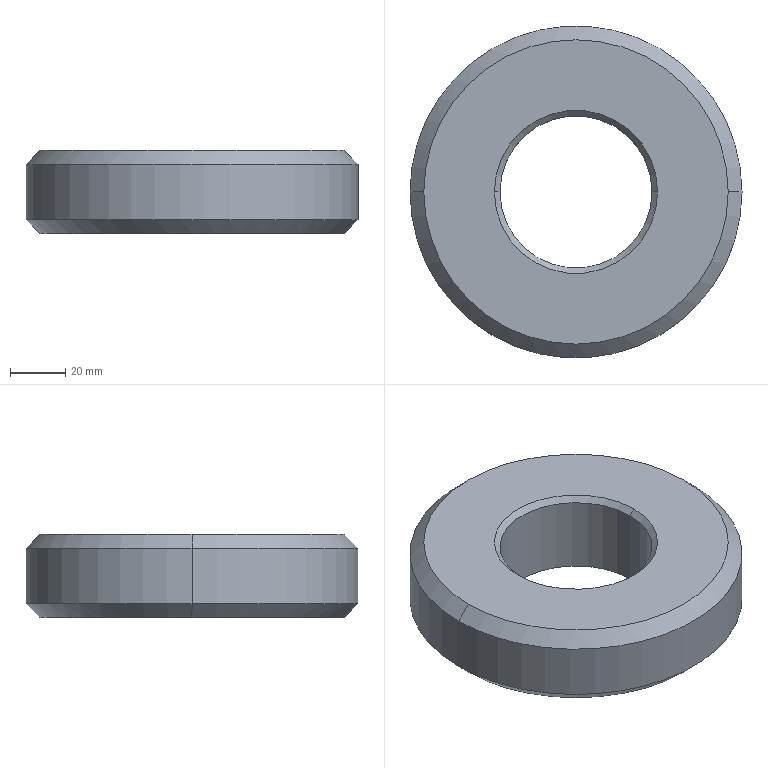Part | SolidWorks | features Chamfer 2, Extrusion 1 | 1 solid | 12 faces | box 120 x 120 x 30 mm | volume 258500 mm3 | cone 6 | cylinder 4 | plane 2 | commonest cylinder face diameters 55 x2 120 x2
STEP:
#1=CARTESIAN_POINT('',(-27.5,0.,28.));
#2=VERTEX_POINT('',#1);
#3=CARTESIAN_POINT('',(27.5,0.,28.));
#4=VERTEX_POINT('',#3);
#5=CARTESIAN_POINT('',(0.,0.,28.));
#6=DIRECTION('',(0.,0.,1.));
#7=DIRECTION('',(1.,0.,0.));
#8=AXIS2_PLACEMENT_3D('',#5,#6,#7);
#9=CIRCLE('',#8,27.5);
#10=EDGE_CURVE('',#2,#4,#9,.T.);
#11=ORIENTED_EDGE('',*,*,#10,.F.);
#12=CARTESIAN_POINT('',(-29.5,0.,30.));
#13=VERTEX_POINT('',#12);
#14=CARTESIAN_POINT('',(-27.5,0.,28.));
#15=DIRECTION('',(-0.7071,0.,0.7071));
#16=VECTOR('',#15,1000.);
#17=LINE('',#14,#16);
#18=EDGE_CURVE('',#2,#13,#17,.T.);
#19=ORIENTED_EDGE('',*,*,#18,.T.);
#20=CARTESIAN_POINT('',(29.5,0.,30.));
#21=VERTEX_POINT('',#20);
#22=CARTESIAN_POINT('',(0.,0.,30.));
#23=DIRECTION('',(0.,0.,-1.));
#24=DIRECTION('',(1.,0.,0.));
#25=AXIS2_PLACEMENT_3D('',#22,#23,#24);
#26=CIRCLE('',#25,29.5);
#27=EDGE_CURVE('',#21,#13,#26,.T.);
#28=ORIENTED_EDGE('',*,*,#27,.F.);
#29=CARTESIAN_POINT('',(27.5,0.,28.));
#30=DIRECTION('',(0.7071,0.,0.7071));
#31=VECTOR('',#30,1000.);
#32=LINE('',#29,#31);
#33=EDGE_CURVE('',#4,#21,#32,.T.);
#34=ORIENTED_EDGE('',*,*,#33,.F.);
#35=EDGE_LOOP('',(#11,#19,#28,#34));
#36=FACE_OUTER_BOUND('',#35,.T.);
#37=CARTESIAN_POINT('',(0.,0.,28.));
#38=DIRECTION('',(0.,0.,1.));
#39=DIRECTION('',(1.,0.,0.));
#40=AXIS2_PLACEMENT_3D('',#37,#38,#39);
#41=CONICAL_SURFACE('',#40,27.5,0.7854);
#42=ADVANCED_FACE('',(#36),#41,.F.);
#43=CARTESIAN_POINT('',(55.,0.,30.));
#44=VERTEX_POINT('',#43);
#45=CARTESIAN_POINT('',(-55.,0.,30.));
#46=VERTEX_POINT('',#45);
#47=CARTESIAN_POINT('',(0.,0.,30.));
#48=DIRECTION('',(0.,0.,1.));
#49=DIRECTION('',(1.,0.,0.));
#50=AXIS2_PLACEMENT_3D('',#47,#48,#49);
#51=CIRCLE('',#50,55.);
#52=EDGE_CURVE('',#44,#46,#51,.T.);
#53=ORIENTED_EDGE('',*,*,#52,.F.);
#54=CARTESIAN_POINT('',(60.,0.,25.));
#55=VERTEX_POINT('',#54);
#56=CARTESIAN_POINT('',(55.,0.,30.));
#57=DIRECTION('',(0.7071,0.,-0.7071));
#58=VECTOR('',#57,1000.);
#59=LINE('',#56,#58);
#60=EDGE_CURVE('',#44,#55,#59,.T.);
#61=ORIENTED_EDGE('',*,*,#60,.T.);
#62=CARTESIAN_POINT('',(-60.,0.,25.));
#63=VERTEX_POINT('',#62);
#64=CARTESIAN_POINT('',(0.,0.,25.));
#65=DIRECTION('',(0.,0.,-1.));
#66=DIRECTION('',(1.,0.,0.));
#67=AXIS2_PLACEMENT_3D('',#64,#65,#66);
#68=CIRCLE('',#67,60.);
#69=EDGE_CURVE('',#63,#55,#68,.T.);
#70=ORIENTED_EDGE('',*,*,#69,.F.);
#71=CARTESIAN_POINT('',(-55.,0.,30.));
#72=DIRECTION('',(-0.7071,0.,-0.7071));
#73=VECTOR('',#72,1000.);
#74=LINE('',#71,#73);
#75=EDGE_CURVE('',#46,#63,#74,.T.);
#76=ORIENTED_EDGE('',*,*,#75,.F.);
#77=EDGE_LOOP('',(#53,#61,#70,#76));
#78=FACE_OUTER_BOUND('',#77,.T.);
#79=CARTESIAN_POINT('',(0.,0.,30.));
#80=DIRECTION('',(0.,0.,-1.));
#81=DIRECTION('',(-1.,0.,0.));
#82=AXIS2_PLACEMENT_3D('',#79,#80,#81);
#83=CONICAL_SURFACE('',#82,55.,0.7854);
#84=ADVANCED_FACE('',(#78),#83,.T.);
#85=CARTESIAN_POINT('',(-55.,0.,0.));
#86=VERTEX_POINT('',#85);
#87=CARTESIAN_POINT('',(55.,0.,0.));
#88=VERTEX_POINT('',#87);
#89=CARTESIAN_POINT('',(0.,0.,0.));
#90=DIRECTION('',(0.,0.,-1.));
#91=DIRECTION('',(1.,0.,0.));
#92=AXIS2_PLACEMENT_3D('',#89,#90,#91);
#93=CIRCLE('',#92,55.);
#94=EDGE_CURVE('',#86,#88,#93,.T.);
#95=ORIENTED_EDGE('',*,*,#94,.F.);
#96=CARTESIAN_POINT('',(-60.,0.,5.));
#97=VERTEX_POINT('',#96);
#98=CARTESIAN_POINT('',(-60.,0.,5.));
#99=DIRECTION('',(-0.7071,0.,0.7071));
#100=VECTOR('',#99,1000.);
#101=LINE('',#98,#100);
#102=EDGE_CURVE('',#86,#97,#101,.T.);
#103=ORIENTED_EDGE('',*,*,#102,.T.);
#104=CARTESIAN_POINT('',(60.,0.,5.));
#105=VERTEX_POINT('',#104);
#106=CARTESIAN_POINT('',(0.,0.,5.));
#107=DIRECTION('',(0.,0.,1.));
#108=DIRECTION('',(1.,0.,0.));
#109=AXIS2_PLACEMENT_3D('',#106,#107,#108);
#110=CIRCLE('',#109,60.);
#111=EDGE_CURVE('',#105,#97,#110,.T.);
#112=ORIENTED_EDGE('',*,*,#111,.F.);
#113=CARTESIAN_POINT('',(60.,0.,5.));
#114=DIRECTION('',(0.7071,0.,0.7071));
#115=VECTOR('',#114,1000.);
#116=LINE('',#113,#115);
#117=EDGE_CURVE('',#88,#105,#116,.T.);
#118=ORIENTED_EDGE('',*,*,#117,.F.);
#119=EDGE_LOOP('',(#95,#103,#112,#118));
#120=FACE_OUTER_BOUND('',#119,.T.);
#121=CARTESIAN_POINT('',(0.,0.,5.));
#122=DIRECTION('',(0.,0.,1.));
#123=DIRECTION('',(1.,0.,0.));
#124=AXIS2_PLACEMENT_3D('',#121,#122,#123);
#125=CONICAL_SURFACE('',#124,60.,0.7854);
#126=ADVANCED_FACE('',(#120),#125,.T.);
#127=ORIENTED_EDGE('',*,*,#10,.T.);
#128=CARTESIAN_POINT('',(27.5,0.,0.));
#129=VERTEX_POINT('',#128);
#130=CARTESIAN_POINT('',(27.5,0.,30.));
#131=DIRECTION('',(0.,0.,-1.));
#132=VECTOR('',#131,1000.);
#133=LINE('',#130,#132);
#134=EDGE_CURVE('',#4,#129,#133,.T.);
#135=ORIENTED_EDGE('',*,*,#134,.T.);
#136=CARTESIAN_POINT('',(-27.5,0.,0.));
#137=VERTEX_POINT('',#136);
#138=CARTESIAN_POINT('',(0.,0.,0.));
#139=DIRECTION('',(0.,0.,1.));
#140=DIRECTION('',(1.,0.,0.));
#141=AXIS2_PLACEMENT_3D('',#138,#139,#140);
#142=CIRCLE('',#141,27.5);
#143=EDGE_CURVE('',#137,#129,#142,.T.);
#144=ORIENTED_EDGE('',*,*,#143,.F.);
#145=CARTESIAN_POINT('',(-27.5,0.,30.));
#146=DIRECTION('',(0.,0.,-1.));
#147=VECTOR('',#146,1000.);
#148=LINE('',#145,#147);
#149=EDGE_CURVE('',#2,#137,#148,.T.);
#150=ORIENTED_EDGE('',*,*,#149,.F.);
#151=EDGE_LOOP('',(#127,#135,#144,#150));
#152=FACE_OUTER_BOUND('',#151,.T.);
#153=CARTESIAN_POINT('',(0.,0.,30.));
#154=DIRECTION('',(0.,0.,-1.));
#155=DIRECTION('',(-1.,0.,0.));
#156=AXIS2_PLACEMENT_3D('',#153,#154,#155);
#157=CYLINDRICAL_SURFACE('',#156,27.5);
#158=ADVANCED_FACE('',(#152),#157,.F.);
#159=ORIENTED_EDGE('',*,*,#69,.T.);
#160=CARTESIAN_POINT('',(60.,0.,30.));
#161=DIRECTION('',(0.,0.,-1.));
#162=VECTOR('',#161,1000.);
#163=LINE('',#160,#162);
#164=EDGE_CURVE('',#55,#105,#163,.T.);
#165=ORIENTED_EDGE('',*,*,#164,.T.);
#166=ORIENTED_EDGE('',*,*,#111,.T.);
#167=CARTESIAN_POINT('',(-60.,0.,30.));
#168=DIRECTION('',(0.,0.,-1.));
#169=VECTOR('',#168,1000.);
#170=LINE('',#167,#169);
#171=EDGE_CURVE('',#63,#97,#170,.T.);
#172=ORIENTED_EDGE('',*,*,#171,.F.);
#173=EDGE_LOOP('',(#159,#165,#166,#172));
#174=FACE_OUTER_BOUND('',#173,.T.);
#175=CARTESIAN_POINT('',(0.,0.,30.));
#176=DIRECTION('',(0.,0.,-1.));
#177=DIRECTION('',(-1.,0.,0.));
#178=AXIS2_PLACEMENT_3D('',#175,#176,#177);
#179=CYLINDRICAL_SURFACE('',#178,60.);
#180=ADVANCED_FACE('',(#174),#179,.T.);
#181=ORIENTED_EDGE('',*,*,#27,.T.);
#182=CARTESIAN_POINT('',(0.,0.,30.));
#183=DIRECTION('',(0.,0.,-1.));
#184=DIRECTION('',(1.,0.,0.));
#185=AXIS2_PLACEMENT_3D('',#182,#183,#184);
#186=CIRCLE('',#185,29.5);
#187=EDGE_CURVE('',#13,#21,#186,.T.);
#188=ORIENTED_EDGE('',*,*,#187,.T.);
#189=EDGE_LOOP('',(#181,#188));
#190=FACE_BOUND('',#189,.T.);
#191=CARTESIAN_POINT('',(0.,0.,30.));
#192=DIRECTION('',(0.,0.,1.));
#193=DIRECTION('',(1.,0.,0.));
#194=AXIS2_PLACEMENT_3D('',#191,#192,#193);
#195=CIRCLE('',#194,55.);
#196=EDGE_CURVE('',#46,#44,#195,.T.);
#197=ORIENTED_EDGE('',*,*,#196,.T.);
#198=ORIENTED_EDGE('',*,*,#52,.T.);
#199=EDGE_LOOP('',(#197,#198));
#200=FACE_OUTER_BOUND('',#199,.T.);
#201=CARTESIAN_POINT('',(0.,0.,30.));
#202=DIRECTION('',(0.,0.,1.));
#203=DIRECTION('',(1.,0.,0.));
#204=AXIS2_PLACEMENT_3D('',#201,#202,#203);
#205=PLANE('',#204);
#206=ADVANCED_FACE('',(#190,#200),#205,.T.);
#207=CARTESIAN_POINT('',(0.,0.,0.));
#208=DIRECTION('',(0.,0.,-1.));
#209=DIRECTION('',(1.,0.,0.));
#210=AXIS2_PLACEMENT_3D('',#207,#208,#209);
#211=CIRCLE('',#210,55.);
#212=EDGE_CURVE('',#88,#86,#211,.T.);
#213=ORIENTED_EDGE('',*,*,#212,.T.);
#214=ORIENTED_EDGE('',*,*,#94,.T.);
#215=EDGE_LOOP('',(#213,#214));
#216=FACE_OUTER_BOUND('',#215,.T.);
#217=ORIENTED_EDGE('',*,*,#143,.T.);
#218=CARTESIAN_POINT('',(0.,0.,0.));
#219=DIRECTION('',(0.,0.,1.));
#220=DIRECTION('',(1.,0.,0.));
#221=AXIS2_PLACEMENT_3D('',#218,#219,#220);
#222=CIRCLE('',#221,27.5);
#223=EDGE_CURVE('',#129,#137,#222,.T.);
#224=ORIENTED_EDGE('',*,*,#223,.T.);
#225=EDGE_LOOP('',(#217,#224));
#226=FACE_BOUND('',#225,.T.);
#227=CARTESIAN_POINT('',(0.,0.,0.));
#228=DIRECTION('',(0.,0.,1.));
#229=DIRECTION('',(1.,0.,0.));
#230=AXIS2_PLACEMENT_3D('',#227,#228,#229);
#231=PLANE('',#230);
#232=ADVANCED_FACE('',(#216,#226),#231,.F.);
#233=ORIENTED_EDGE('',*,*,#164,.F.);
#234=CARTESIAN_POINT('',(0.,0.,25.));
#235=DIRECTION('',(0.,0.,-1.));
#236=DIRECTION('',(1.,0.,0.));
#237=AXIS2_PLACEMENT_3D('',#234,#235,#236);
#238=CIRCLE('',#237,60.);
#239=EDGE_CURVE('',#55,#63,#238,.T.);
#240=ORIENTED_EDGE('',*,*,#239,.T.);
#241=ORIENTED_EDGE('',*,*,#171,.T.);
#242=CARTESIAN_POINT('',(0.,0.,5.));
#243=DIRECTION('',(0.,0.,1.));
#244=DIRECTION('',(1.,0.,0.));
#245=AXIS2_PLACEMENT_3D('',#242,#243,#244);
#246=CIRCLE('',#245,60.);
#247=EDGE_CURVE('',#97,#105,#246,.T.);
#248=ORIENTED_EDGE('',*,*,#247,.T.);
#249=EDGE_LOOP('',(#233,#240,#241,#248));
#250=FACE_OUTER_BOUND('',#249,.T.);
#251=CARTESIAN_POINT('',(0.,0.,30.));
#252=DIRECTION('',(0.,0.,-1.));
#253=DIRECTION('',(-1.,0.,0.));
#254=AXIS2_PLACEMENT_3D('',#251,#252,#253);
#255=CYLINDRICAL_SURFACE('',#254,60.);
#256=ADVANCED_FACE('',(#250),#255,.T.);
#257=ORIENTED_EDGE('',*,*,#134,.F.);
#258=CARTESIAN_POINT('',(0.,0.,28.));
#259=DIRECTION('',(0.,0.,1.));
#260=DIRECTION('',(1.,0.,0.));
#261=AXIS2_PLACEMENT_3D('',#258,#259,#260);
#262=CIRCLE('',#261,27.5);
#263=EDGE_CURVE('',#4,#2,#262,.T.);
#264=ORIENTED_EDGE('',*,*,#263,.T.);
#265=ORIENTED_EDGE('',*,*,#149,.T.);
#266=ORIENTED_EDGE('',*,*,#223,.F.);
#267=EDGE_LOOP('',(#257,#264,#265,#266));
#268=FACE_OUTER_BOUND('',#267,.T.);
#269=CARTESIAN_POINT('',(0.,0.,30.));
#270=DIRECTION('',(0.,0.,-1.));
#271=DIRECTION('',(-1.,0.,0.));
#272=AXIS2_PLACEMENT_3D('',#269,#270,#271);
#273=CYLINDRICAL_SURFACE('',#272,27.5);
#274=ADVANCED_FACE('',(#268),#273,.F.);
#275=ORIENTED_EDGE('',*,*,#102,.F.);
#276=ORIENTED_EDGE('',*,*,#212,.F.);
#277=ORIENTED_EDGE('',*,*,#117,.T.);
#278=ORIENTED_EDGE('',*,*,#247,.F.);
#279=EDGE_LOOP('',(#275,#276,#277,#278));
#280=FACE_OUTER_BOUND('',#279,.T.);
#281=CARTESIAN_POINT('',(0.,0.,5.));
#282=DIRECTION('',(0.,0.,1.));
#283=DIRECTION('',(1.,0.,0.));
#284=AXIS2_PLACEMENT_3D('',#281,#282,#283);
#285=CONICAL_SURFACE('',#284,60.,0.7854);
#286=ADVANCED_FACE('',(#280),#285,.T.);
#287=ORIENTED_EDGE('',*,*,#60,.F.);
#288=ORIENTED_EDGE('',*,*,#196,.F.);
#289=ORIENTED_EDGE('',*,*,#75,.T.);
#290=ORIENTED_EDGE('',*,*,#239,.F.);
#291=EDGE_LOOP('',(#287,#288,#289,#290));
#292=FACE_OUTER_BOUND('',#291,.T.);
#293=CARTESIAN_POINT('',(0.,0.,30.));
#294=DIRECTION('',(0.,0.,-1.));
#295=DIRECTION('',(-1.,0.,0.));
#296=AXIS2_PLACEMENT_3D('',#293,#294,#295);
#297=CONICAL_SURFACE('',#296,55.,0.7854);
#298=ADVANCED_FACE('',(#292),#297,.T.);
#299=ORIENTED_EDGE('',*,*,#18,.F.);
#300=ORIENTED_EDGE('',*,*,#263,.F.);
#301=ORIENTED_EDGE('',*,*,#33,.T.);
#302=ORIENTED_EDGE('',*,*,#187,.F.);
#303=EDGE_LOOP('',(#299,#300,#301,#302));
#304=FACE_OUTER_BOUND('',#303,.T.);
#305=CARTESIAN_POINT('',(0.,0.,28.));
#306=DIRECTION('',(0.,0.,1.));
#307=DIRECTION('',(1.,0.,0.));
#308=AXIS2_PLACEMENT_3D('',#305,#306,#307);
#309=CONICAL_SURFACE('',#308,27.5,0.7854);
#310=ADVANCED_FACE('',(#304),#309,.F.);
#311=CLOSED_SHELL('',(#42,#84,#126,#158,#180,#206,#232,#256,#274,#286,#298,#310));
#312=MANIFOLD_SOLID_BREP('',#311);
#313=CARTESIAN_POINT('',(0.,0.,0.));
#314=DIRECTION('',(0.,0.,1.));
#315=DIRECTION('',(1.,0.,0.));
#316=AXIS2_PLACEMENT_3D('',#313,#314,#315);
#317=(LENGTH_UNIT()NAMED_UNIT(*)SI_UNIT(.MILLI.,.METRE.));
#318=UNCERTAINTY_MEASURE_WITH_UNIT(LENGTH_MEASURE(0.00001),#317,'','');
#319=(NAMED_UNIT(*)PLANE_ANGLE_UNIT()SI_UNIT($,.RADIAN.));
#320=(NAMED_UNIT(*)SI_UNIT($,.STERADIAN.)SOLID_ANGLE_UNIT());
#321=(GEOMETRIC_REPRESENTATION_CONTEXT(3)GLOBAL_UNCERTAINTY_ASSIGNED_CONTEXT((#318))GLOBAL_UNIT_ASSIGNED_CONTEXT((#317,#319,#320))REPRESENTATION_CONTEXT('',''));
#322=ADVANCED_BREP_SHAPE_REPRESENTATION('',(#312,#316),#321);